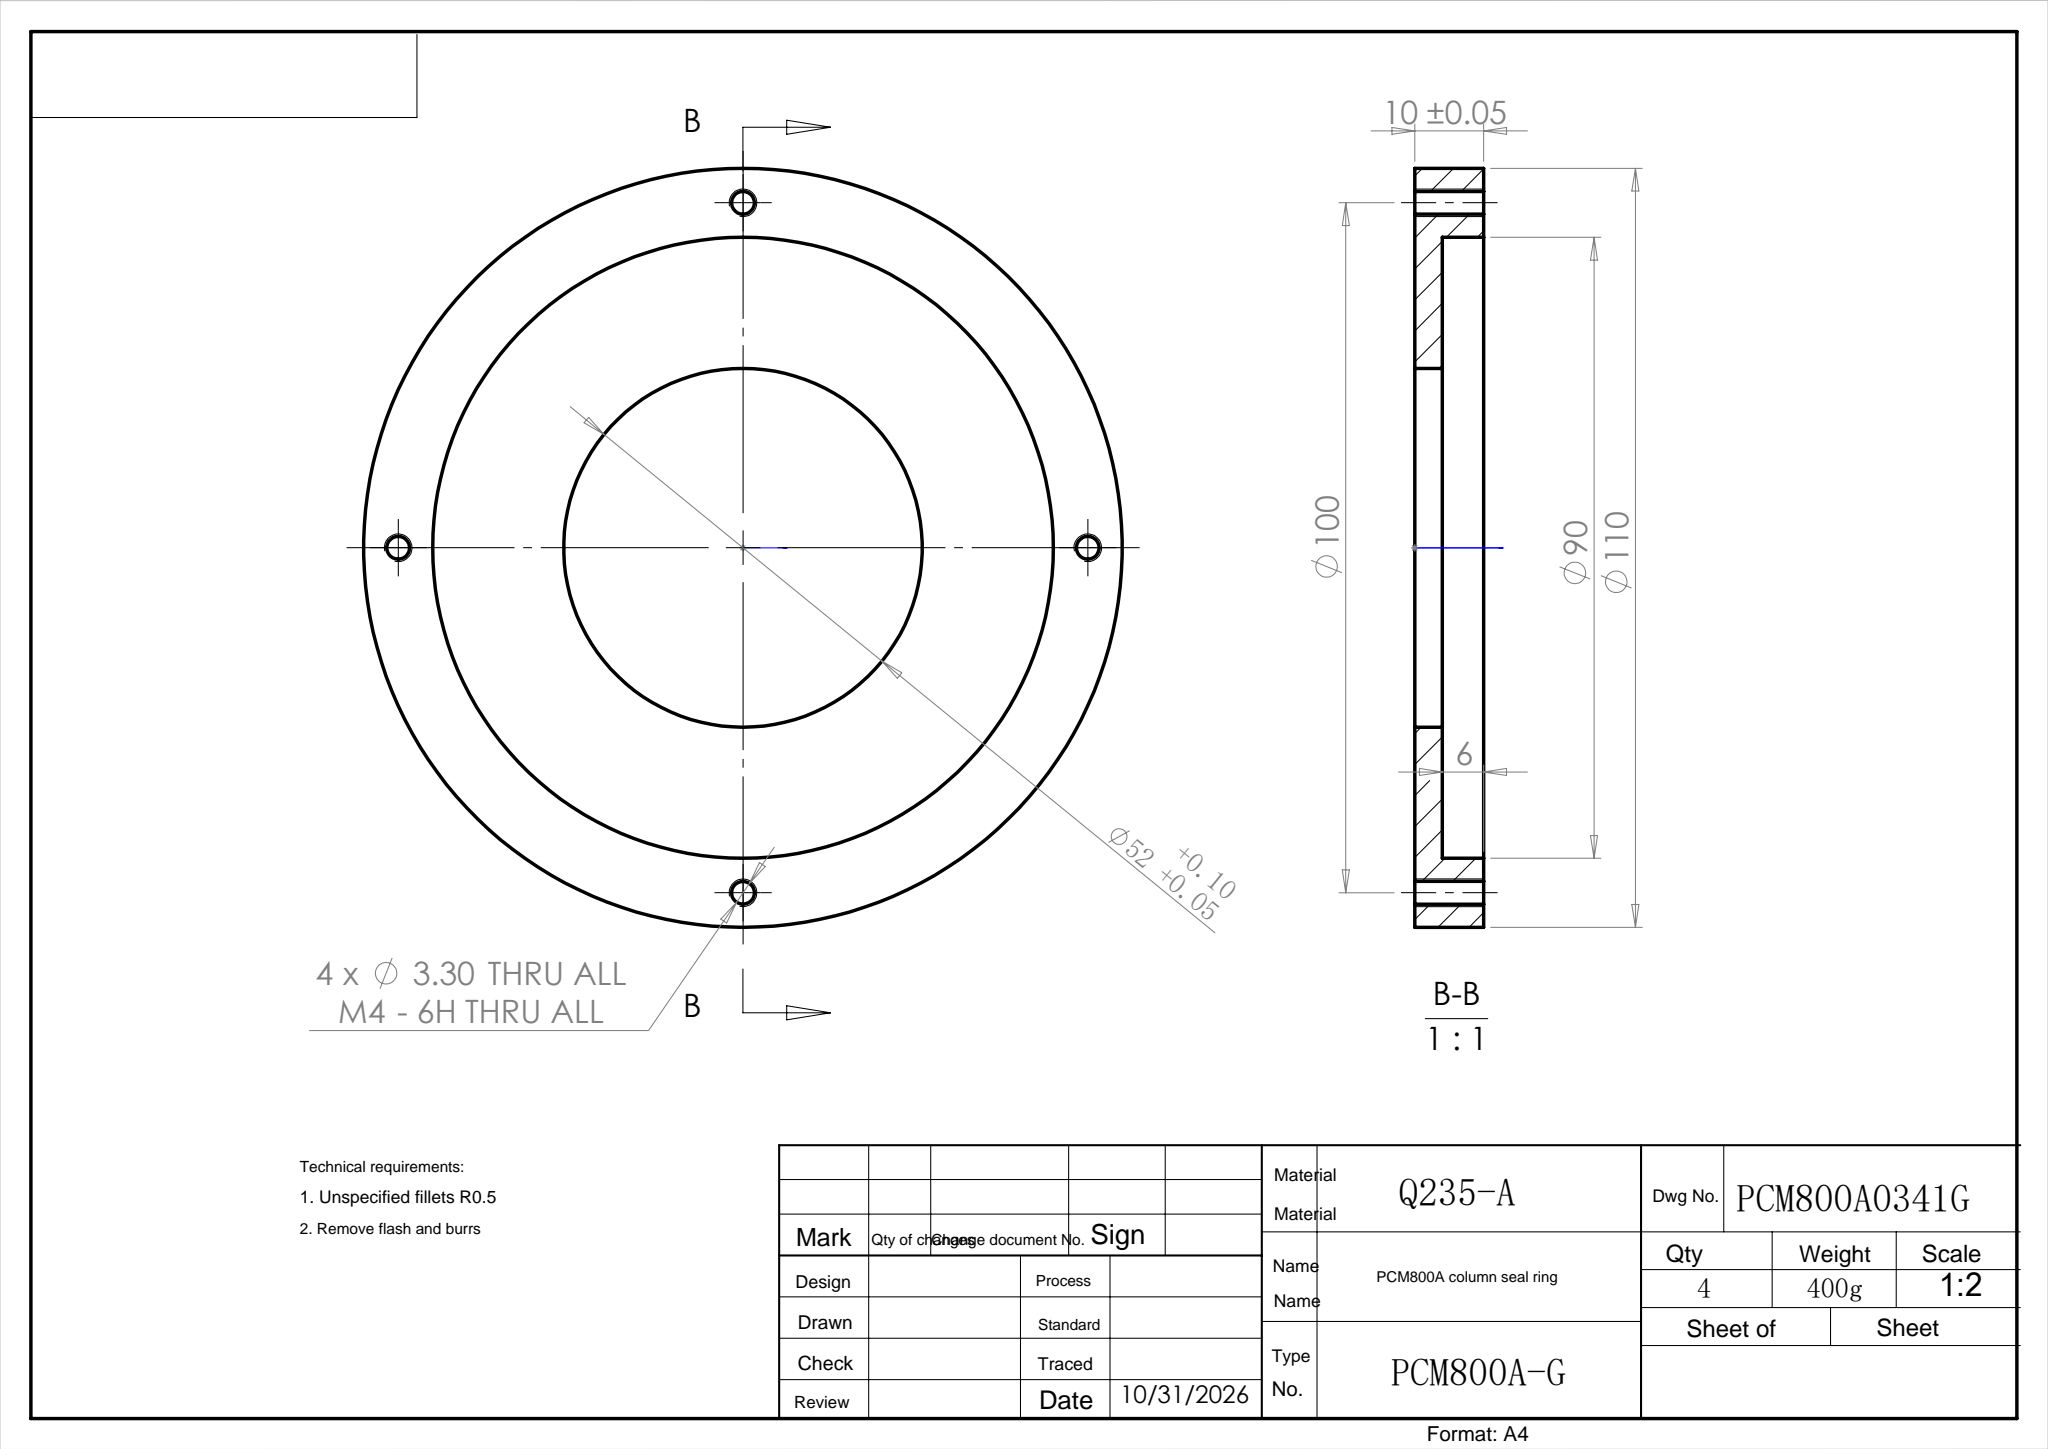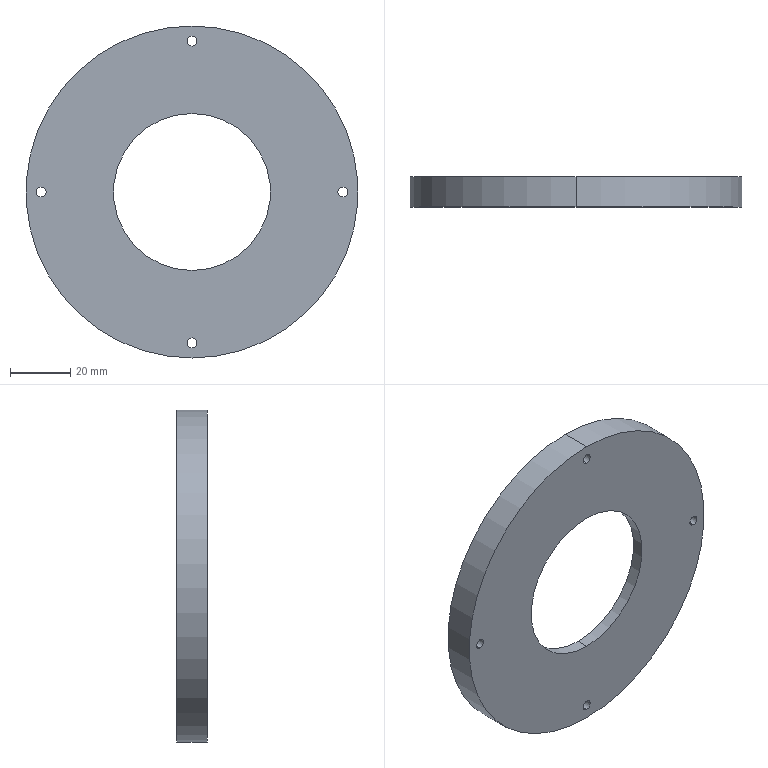Part | SolidWorks | features HoleWzd 1, Revolution 1 | 1 solid | 17 faces | box 110 x 10 x 110 mm | volume 48026 mm3 | cylinder 14 | plane 3 | commonest cylinder face diameters 3.3 x8 52 x2 90 x2 110 x2
STEP:
#1=CARTESIAN_POINT('',(-50.,0.,-1.65));
#2=VERTEX_POINT('',#1);
#3=CARTESIAN_POINT('',(-50.,0.,1.65));
#4=VERTEX_POINT('',#3);
#5=CARTESIAN_POINT('',(-50.,0.,0.));
#6=DIRECTION('',(0.,1.,0.));
#7=DIRECTION('',(0.,0.,1.));
#8=AXIS2_PLACEMENT_3D('',#5,#6,#7);
#9=CIRCLE('',#8,1.65);
#10=EDGE_CURVE('',#2,#4,#9,.T.);
#11=ORIENTED_EDGE('',*,*,#10,.F.);
#12=CARTESIAN_POINT('',(-50.,10.,-1.65));
#13=VERTEX_POINT('',#12);
#14=CARTESIAN_POINT('',(-50.,10.,-1.65));
#15=DIRECTION('',(0.,1.,0.));
#16=VECTOR('',#15,1000.);
#17=LINE('',#14,#16);
#18=EDGE_CURVE('',#2,#13,#17,.T.);
#19=ORIENTED_EDGE('',*,*,#18,.T.);
#20=CARTESIAN_POINT('',(-50.,10.,1.65));
#21=VERTEX_POINT('',#20);
#22=CARTESIAN_POINT('',(-50.,10.,0.));
#23=DIRECTION('',(0.,1.,0.));
#24=DIRECTION('',(0.,0.,1.));
#25=AXIS2_PLACEMENT_3D('',#22,#23,#24);
#26=CIRCLE('',#25,1.65);
#27=EDGE_CURVE('',#13,#21,#26,.T.);
#28=ORIENTED_EDGE('',*,*,#27,.T.);
#29=CARTESIAN_POINT('',(-50.,10.,1.65));
#30=DIRECTION('',(0.,1.,0.));
#31=VECTOR('',#30,1000.);
#32=LINE('',#29,#31);
#33=EDGE_CURVE('',#4,#21,#32,.T.);
#34=ORIENTED_EDGE('',*,*,#33,.F.);
#35=EDGE_LOOP('',(#11,#19,#28,#34));
#36=FACE_OUTER_BOUND('',#35,.T.);
#37=CARTESIAN_POINT('',(-50.,10.,0.));
#38=DIRECTION('',(0.,1.,0.));
#39=DIRECTION('',(0.,0.,1.));
#40=AXIS2_PLACEMENT_3D('',#37,#38,#39);
#41=CYLINDRICAL_SURFACE('',#40,1.65);
#42=ADVANCED_FACE('',(#36),#41,.F.);
#43=CARTESIAN_POINT('',(0.,0.,-51.65));
#44=VERTEX_POINT('',#43);
#45=CARTESIAN_POINT('',(0.,0.,-48.35));
#46=VERTEX_POINT('',#45);
#47=CARTESIAN_POINT('',(0.,0.,-50.));
#48=DIRECTION('',(0.,1.,0.));
#49=DIRECTION('',(0.,0.,1.));
#50=AXIS2_PLACEMENT_3D('',#47,#48,#49);
#51=CIRCLE('',#50,1.65);
#52=EDGE_CURVE('',#44,#46,#51,.T.);
#53=ORIENTED_EDGE('',*,*,#52,.F.);
#54=CARTESIAN_POINT('',(0.,10.,-51.65));
#55=VERTEX_POINT('',#54);
#56=CARTESIAN_POINT('',(0.,10.,-51.65));
#57=DIRECTION('',(0.,1.,0.));
#58=VECTOR('',#57,1000.);
#59=LINE('',#56,#58);
#60=EDGE_CURVE('',#44,#55,#59,.T.);
#61=ORIENTED_EDGE('',*,*,#60,.T.);
#62=CARTESIAN_POINT('',(0.,10.,-48.35));
#63=VERTEX_POINT('',#62);
#64=CARTESIAN_POINT('',(0.,10.,-50.));
#65=DIRECTION('',(0.,1.,0.));
#66=DIRECTION('',(0.,0.,1.));
#67=AXIS2_PLACEMENT_3D('',#64,#65,#66);
#68=CIRCLE('',#67,1.65);
#69=EDGE_CURVE('',#55,#63,#68,.T.);
#70=ORIENTED_EDGE('',*,*,#69,.T.);
#71=CARTESIAN_POINT('',(0.,10.,-48.35));
#72=DIRECTION('',(0.,1.,0.));
#73=VECTOR('',#72,1000.);
#74=LINE('',#71,#73);
#75=EDGE_CURVE('',#46,#63,#74,.T.);
#76=ORIENTED_EDGE('',*,*,#75,.F.);
#77=EDGE_LOOP('',(#53,#61,#70,#76));
#78=FACE_OUTER_BOUND('',#77,.T.);
#79=CARTESIAN_POINT('',(0.,10.,-50.));
#80=DIRECTION('',(0.,1.,0.));
#81=DIRECTION('',(0.,0.,1.));
#82=AXIS2_PLACEMENT_3D('',#79,#80,#81);
#83=CYLINDRICAL_SURFACE('',#82,1.65);
#84=ADVANCED_FACE('',(#78),#83,.F.);
#85=CARTESIAN_POINT('',(50.,0.,-1.65));
#86=VERTEX_POINT('',#85);
#87=CARTESIAN_POINT('',(50.,0.,1.65));
#88=VERTEX_POINT('',#87);
#89=CARTESIAN_POINT('',(50.,0.,0.));
#90=DIRECTION('',(0.,1.,0.));
#91=DIRECTION('',(0.,0.,1.));
#92=AXIS2_PLACEMENT_3D('',#89,#90,#91);
#93=CIRCLE('',#92,1.65);
#94=EDGE_CURVE('',#86,#88,#93,.T.);
#95=ORIENTED_EDGE('',*,*,#94,.F.);
#96=CARTESIAN_POINT('',(50.,10.,-1.65));
#97=VERTEX_POINT('',#96);
#98=CARTESIAN_POINT('',(50.,10.,-1.65));
#99=DIRECTION('',(0.,1.,0.));
#100=VECTOR('',#99,1000.);
#101=LINE('',#98,#100);
#102=EDGE_CURVE('',#86,#97,#101,.T.);
#103=ORIENTED_EDGE('',*,*,#102,.T.);
#104=CARTESIAN_POINT('',(50.,10.,1.65));
#105=VERTEX_POINT('',#104);
#106=CARTESIAN_POINT('',(50.,10.,0.));
#107=DIRECTION('',(0.,1.,0.));
#108=DIRECTION('',(0.,0.,1.));
#109=AXIS2_PLACEMENT_3D('',#106,#107,#108);
#110=CIRCLE('',#109,1.65);
#111=EDGE_CURVE('',#97,#105,#110,.T.);
#112=ORIENTED_EDGE('',*,*,#111,.T.);
#113=CARTESIAN_POINT('',(50.,10.,1.65));
#114=DIRECTION('',(0.,1.,0.));
#115=VECTOR('',#114,1000.);
#116=LINE('',#113,#115);
#117=EDGE_CURVE('',#88,#105,#116,.T.);
#118=ORIENTED_EDGE('',*,*,#117,.F.);
#119=EDGE_LOOP('',(#95,#103,#112,#118));
#120=FACE_OUTER_BOUND('',#119,.T.);
#121=CARTESIAN_POINT('',(50.,10.,0.));
#122=DIRECTION('',(0.,1.,0.));
#123=DIRECTION('',(0.,0.,1.));
#124=AXIS2_PLACEMENT_3D('',#121,#122,#123);
#125=CYLINDRICAL_SURFACE('',#124,1.65);
#126=ADVANCED_FACE('',(#120),#125,.F.);
#127=CARTESIAN_POINT('',(0.,0.,48.35));
#128=VERTEX_POINT('',#127);
#129=CARTESIAN_POINT('',(0.,0.,51.65));
#130=VERTEX_POINT('',#129);
#131=CARTESIAN_POINT('',(0.,0.,50.));
#132=DIRECTION('',(0.,1.,0.));
#133=DIRECTION('',(0.,0.,1.));
#134=AXIS2_PLACEMENT_3D('',#131,#132,#133);
#135=CIRCLE('',#134,1.65);
#136=EDGE_CURVE('',#128,#130,#135,.T.);
#137=ORIENTED_EDGE('',*,*,#136,.F.);
#138=CARTESIAN_POINT('',(0.,10.,48.35));
#139=VERTEX_POINT('',#138);
#140=CARTESIAN_POINT('',(0.,10.,48.35));
#141=DIRECTION('',(0.,1.,0.));
#142=VECTOR('',#141,1000.);
#143=LINE('',#140,#142);
#144=EDGE_CURVE('',#128,#139,#143,.T.);
#145=ORIENTED_EDGE('',*,*,#144,.T.);
#146=CARTESIAN_POINT('',(0.,10.,51.65));
#147=VERTEX_POINT('',#146);
#148=CARTESIAN_POINT('',(0.,10.,50.));
#149=DIRECTION('',(0.,1.,0.));
#150=DIRECTION('',(0.,0.,1.));
#151=AXIS2_PLACEMENT_3D('',#148,#149,#150);
#152=CIRCLE('',#151,1.65);
#153=EDGE_CURVE('',#139,#147,#152,.T.);
#154=ORIENTED_EDGE('',*,*,#153,.T.);
#155=CARTESIAN_POINT('',(0.,10.,51.65));
#156=DIRECTION('',(0.,1.,0.));
#157=VECTOR('',#156,1000.);
#158=LINE('',#155,#157);
#159=EDGE_CURVE('',#130,#147,#158,.T.);
#160=ORIENTED_EDGE('',*,*,#159,.F.);
#161=EDGE_LOOP('',(#137,#145,#154,#160));
#162=FACE_OUTER_BOUND('',#161,.T.);
#163=CARTESIAN_POINT('',(0.,10.,50.));
#164=DIRECTION('',(0.,1.,0.));
#165=DIRECTION('',(0.,0.,1.));
#166=AXIS2_PLACEMENT_3D('',#163,#164,#165);
#167=CYLINDRICAL_SURFACE('',#166,1.65);
#168=ADVANCED_FACE('',(#162),#167,.F.);
#169=CARTESIAN_POINT('',(0.,10.,-55.));
#170=VERTEX_POINT('',#169);
#171=CARTESIAN_POINT('',(0.,10.,55.));
#172=VERTEX_POINT('',#171);
#173=CARTESIAN_POINT('',(0.,10.,0.));
#174=DIRECTION('',(0.,-1.,0.));
#175=DIRECTION('',(0.,0.,-1.));
#176=AXIS2_PLACEMENT_3D('',#173,#174,#175);
#177=CIRCLE('',#176,55.);
#178=EDGE_CURVE('',#170,#172,#177,.T.);
#179=ORIENTED_EDGE('',*,*,#178,.T.);
#180=CARTESIAN_POINT('',(0.,0.,55.));
#181=VERTEX_POINT('',#180);
#182=CARTESIAN_POINT('',(0.,0.,55.));
#183=DIRECTION('',(0.,-1.,0.));
#184=VECTOR('',#183,1000.);
#185=LINE('',#182,#184);
#186=EDGE_CURVE('',#172,#181,#185,.T.);
#187=ORIENTED_EDGE('',*,*,#186,.T.);
#188=CARTESIAN_POINT('',(0.,0.,-55.));
#189=VERTEX_POINT('',#188);
#190=CARTESIAN_POINT('',(0.,0.,0.));
#191=DIRECTION('',(0.,-1.,0.));
#192=DIRECTION('',(0.,0.,-1.));
#193=AXIS2_PLACEMENT_3D('',#190,#191,#192);
#194=CIRCLE('',#193,55.);
#195=EDGE_CURVE('',#189,#181,#194,.T.);
#196=ORIENTED_EDGE('',*,*,#195,.F.);
#197=CARTESIAN_POINT('',(0.,0.,-55.));
#198=DIRECTION('',(0.,-1.,0.));
#199=VECTOR('',#198,1000.);
#200=LINE('',#197,#199);
#201=EDGE_CURVE('',#170,#189,#200,.T.);
#202=ORIENTED_EDGE('',*,*,#201,.F.);
#203=EDGE_LOOP('',(#179,#187,#196,#202));
#204=FACE_OUTER_BOUND('',#203,.T.);
#205=CARTESIAN_POINT('',(0.,0.,0.));
#206=DIRECTION('',(0.,-1.,0.));
#207=DIRECTION('',(0.,0.,-1.));
#208=AXIS2_PLACEMENT_3D('',#205,#206,#207);
#209=CYLINDRICAL_SURFACE('',#208,55.);
#210=ADVANCED_FACE('',(#204),#209,.T.);
#211=CARTESIAN_POINT('',(0.,10.,45.));
#212=VERTEX_POINT('',#211);
#213=CARTESIAN_POINT('',(0.,10.,-45.));
#214=VERTEX_POINT('',#213);
#215=CARTESIAN_POINT('',(0.,10.,0.));
#216=DIRECTION('',(0.,-1.,0.));
#217=DIRECTION('',(0.,0.,-1.));
#218=AXIS2_PLACEMENT_3D('',#215,#216,#217);
#219=CIRCLE('',#218,45.);
#220=EDGE_CURVE('',#212,#214,#219,.T.);
#221=ORIENTED_EDGE('',*,*,#220,.F.);
#222=CARTESIAN_POINT('',(0.,4.,45.));
#223=VERTEX_POINT('',#222);
#224=CARTESIAN_POINT('',(0.,0.,45.));
#225=DIRECTION('',(0.,-1.,0.));
#226=VECTOR('',#225,1000.);
#227=LINE('',#224,#226);
#228=EDGE_CURVE('',#212,#223,#227,.T.);
#229=ORIENTED_EDGE('',*,*,#228,.T.);
#230=CARTESIAN_POINT('',(0.,4.,-45.));
#231=VERTEX_POINT('',#230);
#232=CARTESIAN_POINT('',(0.,4.,0.));
#233=DIRECTION('',(0.,-1.,0.));
#234=DIRECTION('',(0.,0.,-1.));
#235=AXIS2_PLACEMENT_3D('',#232,#233,#234);
#236=CIRCLE('',#235,45.);
#237=EDGE_CURVE('',#223,#231,#236,.T.);
#238=ORIENTED_EDGE('',*,*,#237,.T.);
#239=CARTESIAN_POINT('',(0.,0.,-45.));
#240=DIRECTION('',(0.,-1.,0.));
#241=VECTOR('',#240,1000.);
#242=LINE('',#239,#241);
#243=EDGE_CURVE('',#214,#231,#242,.T.);
#244=ORIENTED_EDGE('',*,*,#243,.F.);
#245=EDGE_LOOP('',(#221,#229,#238,#244));
#246=FACE_OUTER_BOUND('',#245,.T.);
#247=CARTESIAN_POINT('',(0.,0.,0.));
#248=DIRECTION('',(0.,-1.,0.));
#249=DIRECTION('',(0.,0.,-1.));
#250=AXIS2_PLACEMENT_3D('',#247,#248,#249);
#251=CYLINDRICAL_SURFACE('',#250,45.);
#252=ADVANCED_FACE('',(#246),#251,.F.);
#253=CARTESIAN_POINT('',(0.,4.,26.));
#254=VERTEX_POINT('',#253);
#255=CARTESIAN_POINT('',(0.,4.,-26.));
#256=VERTEX_POINT('',#255);
#257=CARTESIAN_POINT('',(0.,4.,0.));
#258=DIRECTION('',(0.,-1.,0.));
#259=DIRECTION('',(0.,0.,-1.));
#260=AXIS2_PLACEMENT_3D('',#257,#258,#259);
#261=CIRCLE('',#260,26.);
#262=EDGE_CURVE('',#254,#256,#261,.T.);
#263=ORIENTED_EDGE('',*,*,#262,.F.);
#264=CARTESIAN_POINT('',(0.,0.,26.));
#265=VERTEX_POINT('',#264);
#266=CARTESIAN_POINT('',(0.,0.,26.));
#267=DIRECTION('',(0.,-1.,0.));
#268=VECTOR('',#267,1000.);
#269=LINE('',#266,#268);
#270=EDGE_CURVE('',#254,#265,#269,.T.);
#271=ORIENTED_EDGE('',*,*,#270,.T.);
#272=CARTESIAN_POINT('',(0.,0.,-26.));
#273=VERTEX_POINT('',#272);
#274=CARTESIAN_POINT('',(0.,0.,0.));
#275=DIRECTION('',(0.,-1.,0.));
#276=DIRECTION('',(0.,0.,-1.));
#277=AXIS2_PLACEMENT_3D('',#274,#275,#276);
#278=CIRCLE('',#277,26.);
#279=EDGE_CURVE('',#265,#273,#278,.T.);
#280=ORIENTED_EDGE('',*,*,#279,.T.);
#281=CARTESIAN_POINT('',(0.,0.,-26.));
#282=DIRECTION('',(0.,-1.,0.));
#283=VECTOR('',#282,1000.);
#284=LINE('',#281,#283);
#285=EDGE_CURVE('',#256,#273,#284,.T.);
#286=ORIENTED_EDGE('',*,*,#285,.F.);
#287=EDGE_LOOP('',(#263,#271,#280,#286));
#288=FACE_OUTER_BOUND('',#287,.T.);
#289=CARTESIAN_POINT('',(0.,0.,0.));
#290=DIRECTION('',(0.,-1.,0.));
#291=DIRECTION('',(0.,0.,-1.));
#292=AXIS2_PLACEMENT_3D('',#289,#290,#291);
#293=CYLINDRICAL_SURFACE('',#292,26.);
#294=ADVANCED_FACE('',(#288),#293,.F.);
#295=CARTESIAN_POINT('',(-50.,0.,0.));
#296=DIRECTION('',(0.,1.,0.));
#297=DIRECTION('',(0.,0.,1.));
#298=AXIS2_PLACEMENT_3D('',#295,#296,#297);
#299=CIRCLE('',#298,1.65);
#300=EDGE_CURVE('',#4,#2,#299,.T.);
#301=ORIENTED_EDGE('',*,*,#300,.T.);
#302=ORIENTED_EDGE('',*,*,#10,.T.);
#303=EDGE_LOOP('',(#301,#302));
#304=FACE_BOUND('',#303,.T.);
#305=CARTESIAN_POINT('',(0.,0.,-50.));
#306=DIRECTION('',(0.,1.,0.));
#307=DIRECTION('',(0.,0.,1.));
#308=AXIS2_PLACEMENT_3D('',#305,#306,#307);
#309=CIRCLE('',#308,1.65);
#310=EDGE_CURVE('',#46,#44,#309,.T.);
#311=ORIENTED_EDGE('',*,*,#310,.T.);
#312=ORIENTED_EDGE('',*,*,#52,.T.);
#313=EDGE_LOOP('',(#311,#312));
#314=FACE_BOUND('',#313,.T.);
#315=CARTESIAN_POINT('',(50.,0.,0.));
#316=DIRECTION('',(0.,1.,0.));
#317=DIRECTION('',(0.,0.,1.));
#318=AXIS2_PLACEMENT_3D('',#315,#316,#317);
#319=CIRCLE('',#318,1.65);
#320=EDGE_CURVE('',#88,#86,#319,.T.);
#321=ORIENTED_EDGE('',*,*,#320,.T.);
#322=ORIENTED_EDGE('',*,*,#94,.T.);
#323=EDGE_LOOP('',(#321,#322));
#324=FACE_BOUND('',#323,.T.);
#325=CARTESIAN_POINT('',(0.,0.,50.));
#326=DIRECTION('',(0.,1.,0.));
#327=DIRECTION('',(0.,0.,1.));
#328=AXIS2_PLACEMENT_3D('',#325,#326,#327);
#329=CIRCLE('',#328,1.65);
#330=EDGE_CURVE('',#130,#128,#329,.T.);
#331=ORIENTED_EDGE('',*,*,#330,.T.);
#332=ORIENTED_EDGE('',*,*,#136,.T.);
#333=EDGE_LOOP('',(#331,#332));
#334=FACE_BOUND('',#333,.T.);
#335=ORIENTED_EDGE('',*,*,#195,.T.);
#336=CARTESIAN_POINT('',(0.,0.,0.));
#337=DIRECTION('',(0.,-1.,0.));
#338=DIRECTION('',(0.,0.,-1.));
#339=AXIS2_PLACEMENT_3D('',#336,#337,#338);
#340=CIRCLE('',#339,55.);
#341=EDGE_CURVE('',#181,#189,#340,.T.);
#342=ORIENTED_EDGE('',*,*,#341,.T.);
#343=EDGE_LOOP('',(#335,#342));
#344=FACE_OUTER_BOUND('',#343,.T.);
#345=CARTESIAN_POINT('',(0.,0.,0.));
#346=DIRECTION('',(0.,-1.,0.));
#347=DIRECTION('',(0.,0.,-1.));
#348=AXIS2_PLACEMENT_3D('',#345,#346,#347);
#349=CIRCLE('',#348,26.);
#350=EDGE_CURVE('',#273,#265,#349,.T.);
#351=ORIENTED_EDGE('',*,*,#350,.F.);
#352=ORIENTED_EDGE('',*,*,#279,.F.);
#353=EDGE_LOOP('',(#351,#352));
#354=FACE_BOUND('',#353,.T.);
#355=CARTESIAN_POINT('',(-55.,0.,0.));
#356=DIRECTION('',(0.,-1.,0.));
#357=DIRECTION('',(0.,0.,-1.));
#358=AXIS2_PLACEMENT_3D('',#355,#356,#357);
#359=PLANE('',#358);
#360=ADVANCED_FACE('',(#304,#314,#324,#334,#344,#354),#359,.T.);
#361=ORIENTED_EDGE('',*,*,#270,.F.);
#362=CARTESIAN_POINT('',(0.,4.,0.));
#363=DIRECTION('',(0.,-1.,0.));
#364=DIRECTION('',(0.,0.,-1.));
#365=AXIS2_PLACEMENT_3D('',#362,#363,#364);
#366=CIRCLE('',#365,26.);
#367=EDGE_CURVE('',#256,#254,#366,.T.);
#368=ORIENTED_EDGE('',*,*,#367,.F.);
#369=ORIENTED_EDGE('',*,*,#285,.T.);
#370=ORIENTED_EDGE('',*,*,#350,.T.);
#371=EDGE_LOOP('',(#361,#368,#369,#370));
#372=FACE_OUTER_BOUND('',#371,.T.);
#373=CARTESIAN_POINT('',(0.,0.,0.));
#374=DIRECTION('',(0.,-1.,0.));
#375=DIRECTION('',(0.,0.,-1.));
#376=AXIS2_PLACEMENT_3D('',#373,#374,#375);
#377=CYLINDRICAL_SURFACE('',#376,26.);
#378=ADVANCED_FACE('',(#372),#377,.F.);
#379=ORIENTED_EDGE('',*,*,#367,.T.);
#380=ORIENTED_EDGE('',*,*,#262,.T.);
#381=EDGE_LOOP('',(#379,#380));
#382=FACE_BOUND('',#381,.T.);
#383=CARTESIAN_POINT('',(0.,4.,0.));
#384=DIRECTION('',(0.,-1.,0.));
#385=DIRECTION('',(0.,0.,-1.));
#386=AXIS2_PLACEMENT_3D('',#383,#384,#385);
#387=CIRCLE('',#386,45.);
#388=EDGE_CURVE('',#231,#223,#387,.T.);
#389=ORIENTED_EDGE('',*,*,#388,.F.);
#390=ORIENTED_EDGE('',*,*,#237,.F.);
#391=EDGE_LOOP('',(#389,#390));
#392=FACE_OUTER_BOUND('',#391,.T.);
#393=CARTESIAN_POINT('',(-26.,4.,0.));
#394=DIRECTION('',(0.,1.,0.));
#395=DIRECTION('',(0.,0.,1.));
#396=AXIS2_PLACEMENT_3D('',#393,#394,#395);
#397=PLANE('',#396);
#398=ADVANCED_FACE('',(#382,#392),#397,.T.);
#399=ORIENTED_EDGE('',*,*,#228,.F.);
#400=CARTESIAN_POINT('',(0.,10.,0.));
#401=DIRECTION('',(0.,-1.,0.));
#402=DIRECTION('',(0.,0.,-1.));
#403=AXIS2_PLACEMENT_3D('',#400,#401,#402);
#404=CIRCLE('',#403,45.);
#405=EDGE_CURVE('',#214,#212,#404,.T.);
#406=ORIENTED_EDGE('',*,*,#405,.F.);
#407=ORIENTED_EDGE('',*,*,#243,.T.);
#408=ORIENTED_EDGE('',*,*,#388,.T.);
#409=EDGE_LOOP('',(#399,#406,#407,#408));
#410=FACE_OUTER_BOUND('',#409,.T.);
#411=CARTESIAN_POINT('',(0.,0.,0.));
#412=DIRECTION('',(0.,-1.,0.));
#413=DIRECTION('',(0.,0.,-1.));
#414=AXIS2_PLACEMENT_3D('',#411,#412,#413);
#415=CYLINDRICAL_SURFACE('',#414,45.);
#416=ADVANCED_FACE('',(#410),#415,.F.);
#417=CARTESIAN_POINT('',(-50.,10.,0.));
#418=DIRECTION('',(0.,1.,0.));
#419=DIRECTION('',(0.,0.,1.));
#420=AXIS2_PLACEMENT_3D('',#417,#418,#419);
#421=CIRCLE('',#420,1.65);
#422=EDGE_CURVE('',#21,#13,#421,.T.);
#423=ORIENTED_EDGE('',*,*,#422,.F.);
#424=ORIENTED_EDGE('',*,*,#27,.F.);
#425=EDGE_LOOP('',(#423,#424));
#426=FACE_BOUND('',#425,.T.);
#427=CARTESIAN_POINT('',(0.,10.,-50.));
#428=DIRECTION('',(0.,1.,0.));
#429=DIRECTION('',(0.,0.,1.));
#430=AXIS2_PLACEMENT_3D('',#427,#428,#429);
#431=CIRCLE('',#430,1.65);
#432=EDGE_CURVE('',#63,#55,#431,.T.);
#433=ORIENTED_EDGE('',*,*,#432,.F.);
#434=ORIENTED_EDGE('',*,*,#69,.F.);
#435=EDGE_LOOP('',(#433,#434));
#436=FACE_BOUND('',#435,.T.);
#437=CARTESIAN_POINT('',(50.,10.,0.));
#438=DIRECTION('',(0.,1.,0.));
#439=DIRECTION('',(0.,0.,1.));
#440=AXIS2_PLACEMENT_3D('',#437,#438,#439);
#441=CIRCLE('',#440,1.65);
#442=EDGE_CURVE('',#105,#97,#441,.T.);
#443=ORIENTED_EDGE('',*,*,#442,.F.);
#444=ORIENTED_EDGE('',*,*,#111,.F.);
#445=EDGE_LOOP('',(#443,#444));
#446=FACE_BOUND('',#445,.T.);
#447=CARTESIAN_POINT('',(0.,10.,50.));
#448=DIRECTION('',(0.,1.,0.));
#449=DIRECTION('',(0.,0.,1.));
#450=AXIS2_PLACEMENT_3D('',#447,#448,#449);
#451=CIRCLE('',#450,1.65);
#452=EDGE_CURVE('',#147,#139,#451,.T.);
#453=ORIENTED_EDGE('',*,*,#452,.F.);
#454=ORIENTED_EDGE('',*,*,#153,.F.);
#455=EDGE_LOOP('',(#453,#454));
#456=FACE_BOUND('',#455,.T.);
#457=ORIENTED_EDGE('',*,*,#405,.T.);
#458=ORIENTED_EDGE('',*,*,#220,.T.);
#459=EDGE_LOOP('',(#457,#458));
#460=FACE_BOUND('',#459,.T.);
#461=ORIENTED_EDGE('',*,*,#178,.F.);
#462=CARTESIAN_POINT('',(0.,10.,0.));
#463=DIRECTION('',(0.,-1.,0.));
#464=DIRECTION('',(0.,0.,-1.));
#465=AXIS2_PLACEMENT_3D('',#462,#463,#464);
#466=CIRCLE('',#465,55.);
#467=EDGE_CURVE('',#172,#170,#466,.T.);
#468=ORIENTED_EDGE('',*,*,#467,.F.);
#469=EDGE_LOOP('',(#461,#468));
#470=FACE_OUTER_BOUND('',#469,.T.);
#471=CARTESIAN_POINT('',(-45.,10.,0.));
#472=DIRECTION('',(0.,1.,0.));
#473=DIRECTION('',(0.,0.,1.));
#474=AXIS2_PLACEMENT_3D('',#471,#472,#473);
#475=PLANE('',#474);
#476=ADVANCED_FACE('',(#426,#436,#446,#456,#460,#470),#475,.T.);
#477=ORIENTED_EDGE('',*,*,#186,.F.);
#478=ORIENTED_EDGE('',*,*,#467,.T.);
#479=ORIENTED_EDGE('',*,*,#201,.T.);
#480=ORIENTED_EDGE('',*,*,#341,.F.);
#481=EDGE_LOOP('',(#477,#478,#479,#480));
#482=FACE_OUTER_BOUND('',#481,.T.);
#483=CARTESIAN_POINT('',(0.,0.,0.));
#484=DIRECTION('',(0.,-1.,0.));
#485=DIRECTION('',(0.,0.,-1.));
#486=AXIS2_PLACEMENT_3D('',#483,#484,#485);
#487=CYLINDRICAL_SURFACE('',#486,55.);
#488=ADVANCED_FACE('',(#482),#487,.T.);
#489=ORIENTED_EDGE('',*,*,#144,.F.);
#490=ORIENTED_EDGE('',*,*,#330,.F.);
#491=ORIENTED_EDGE('',*,*,#159,.T.);
#492=ORIENTED_EDGE('',*,*,#452,.T.);
#493=EDGE_LOOP('',(#489,#490,#491,#492));
#494=FACE_OUTER_BOUND('',#493,.T.);
#495=CARTESIAN_POINT('',(0.,10.,50.));
#496=DIRECTION('',(0.,1.,0.));
#497=DIRECTION('',(0.,0.,1.));
#498=AXIS2_PLACEMENT_3D('',#495,#496,#497);
#499=CYLINDRICAL_SURFACE('',#498,1.65);
#500=ADVANCED_FACE('',(#494),#499,.F.);
#501=ORIENTED_EDGE('',*,*,#102,.F.);
#502=ORIENTED_EDGE('',*,*,#320,.F.);
#503=ORIENTED_EDGE('',*,*,#117,.T.);
#504=ORIENTED_EDGE('',*,*,#442,.T.);
#505=EDGE_LOOP('',(#501,#502,#503,#504));
#506=FACE_OUTER_BOUND('',#505,.T.);
#507=CARTESIAN_POINT('',(50.,10.,0.));
#508=DIRECTION('',(0.,1.,0.));
#509=DIRECTION('',(0.,0.,1.));
#510=AXIS2_PLACEMENT_3D('',#507,#508,#509);
#511=CYLINDRICAL_SURFACE('',#510,1.65);
#512=ADVANCED_FACE('',(#506),#511,.F.);
#513=ORIENTED_EDGE('',*,*,#60,.F.);
#514=ORIENTED_EDGE('',*,*,#310,.F.);
#515=ORIENTED_EDGE('',*,*,#75,.T.);
#516=ORIENTED_EDGE('',*,*,#432,.T.);
#517=EDGE_LOOP('',(#513,#514,#515,#516));
#518=FACE_OUTER_BOUND('',#517,.T.);
#519=CARTESIAN_POINT('',(0.,10.,-50.));
#520=DIRECTION('',(0.,1.,0.));
#521=DIRECTION('',(0.,0.,1.));
#522=AXIS2_PLACEMENT_3D('',#519,#520,#521);
#523=CYLINDRICAL_SURFACE('',#522,1.65);
#524=ADVANCED_FACE('',(#518),#523,.F.);
#525=ORIENTED_EDGE('',*,*,#18,.F.);
#526=ORIENTED_EDGE('',*,*,#300,.F.);
#527=ORIENTED_EDGE('',*,*,#33,.T.);
#528=ORIENTED_EDGE('',*,*,#422,.T.);
#529=EDGE_LOOP('',(#525,#526,#527,#528));
#530=FACE_OUTER_BOUND('',#529,.T.);
#531=CARTESIAN_POINT('',(-50.,10.,0.));
#532=DIRECTION('',(0.,1.,0.));
#533=DIRECTION('',(0.,0.,1.));
#534=AXIS2_PLACEMENT_3D('',#531,#532,#533);
#535=CYLINDRICAL_SURFACE('',#534,1.65);
#536=ADVANCED_FACE('',(#530),#535,.F.);
#537=CLOSED_SHELL('',(#42,#84,#126,#168,#210,#252,#294,#360,#378,#398,#416,#476,#488,#500,#512,#524,#536));
#538=MANIFOLD_SOLID_BREP('',#537);
#539=CARTESIAN_POINT('',(0.,0.,0.));
#540=DIRECTION('',(0.,0.,1.));
#541=DIRECTION('',(1.,0.,0.));
#542=AXIS2_PLACEMENT_3D('',#539,#540,#541);
#543=(LENGTH_UNIT()NAMED_UNIT(*)SI_UNIT(.MILLI.,.METRE.));
#544=UNCERTAINTY_MEASURE_WITH_UNIT(LENGTH_MEASURE(0.00001),#543,'','');
#545=(NAMED_UNIT(*)PLANE_ANGLE_UNIT()SI_UNIT($,.RADIAN.));
#546=(NAMED_UNIT(*)SI_UNIT($,.STERADIAN.)SOLID_ANGLE_UNIT());
#547=(GEOMETRIC_REPRESENTATION_CONTEXT(3)GLOBAL_UNCERTAINTY_ASSIGNED_CONTEXT((#544))GLOBAL_UNIT_ASSIGNED_CONTEXT((#543,#545,#546))REPRESENTATION_CONTEXT('',''));
#548=ADVANCED_BREP_SHAPE_REPRESENTATION('',(#538,#542),#547);